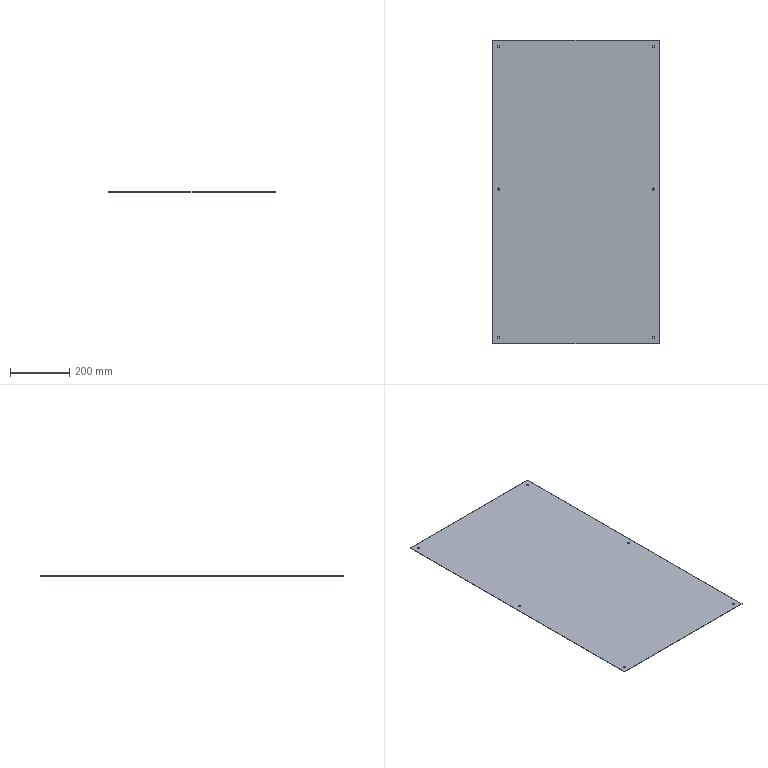Part | SolidWorks | features FlatPattern 1, HoleWzd 1, SMBaseFlange 1, SheetMetal 1 | 1 solid | 18 faces | box 560 x 1020 x 1.2 mm | volume 685163 mm3 | cylinder 12 | plane 6 | commonest cylinder face diameters 7 x12
STEP:
#1=CARTESIAN_POINT('',(16.5,-1000.,0.));
#2=VERTEX_POINT('',#1);
#3=CARTESIAN_POINT('',(23.5,-1000.,0.));
#4=VERTEX_POINT('',#3);
#5=CARTESIAN_POINT('',(20.,-1000.,0.));
#6=DIRECTION('',(0.,0.,1.));
#7=DIRECTION('',(1.,0.,0.));
#8=AXIS2_PLACEMENT_3D('',#5,#6,#7);
#9=CIRCLE('',#8,3.5);
#10=EDGE_CURVE('',#2,#4,#9,.T.);
#11=ORIENTED_EDGE('',*,*,#10,.F.);
#12=CARTESIAN_POINT('',(16.5,-1000.,1.2));
#13=VERTEX_POINT('',#12);
#14=CARTESIAN_POINT('',(16.5,-1000.,1.2));
#15=DIRECTION('',(0.,0.,1.));
#16=VECTOR('',#15,1000.);
#17=LINE('',#14,#16);
#18=EDGE_CURVE('',#2,#13,#17,.T.);
#19=ORIENTED_EDGE('',*,*,#18,.T.);
#20=CARTESIAN_POINT('',(23.5,-1000.,1.2));
#21=VERTEX_POINT('',#20);
#22=CARTESIAN_POINT('',(20.,-1000.,1.2));
#23=DIRECTION('',(0.,0.,1.));
#24=DIRECTION('',(1.,0.,0.));
#25=AXIS2_PLACEMENT_3D('',#22,#23,#24);
#26=CIRCLE('',#25,3.5);
#27=EDGE_CURVE('',#13,#21,#26,.T.);
#28=ORIENTED_EDGE('',*,*,#27,.T.);
#29=CARTESIAN_POINT('',(23.5,-1000.,1.2));
#30=DIRECTION('',(0.,0.,1.));
#31=VECTOR('',#30,1000.);
#32=LINE('',#29,#31);
#33=EDGE_CURVE('',#4,#21,#32,.T.);
#34=ORIENTED_EDGE('',*,*,#33,.F.);
#35=EDGE_LOOP('',(#11,#19,#28,#34));
#36=FACE_OUTER_BOUND('',#35,.T.);
#37=CARTESIAN_POINT('',(20.,-1000.,1.2));
#38=DIRECTION('',(0.,0.,1.));
#39=DIRECTION('',(1.,0.,0.));
#40=AXIS2_PLACEMENT_3D('',#37,#38,#39);
#41=CYLINDRICAL_SURFACE('',#40,3.5);
#42=ADVANCED_FACE('',(#36),#41,.F.);
#43=CARTESIAN_POINT('',(536.5,-1000.,0.));
#44=VERTEX_POINT('',#43);
#45=CARTESIAN_POINT('',(543.5,-1000.,0.));
#46=VERTEX_POINT('',#45);
#47=CARTESIAN_POINT('',(540.,-1000.,0.));
#48=DIRECTION('',(0.,0.,1.));
#49=DIRECTION('',(1.,0.,0.));
#50=AXIS2_PLACEMENT_3D('',#47,#48,#49);
#51=CIRCLE('',#50,3.5);
#52=EDGE_CURVE('',#44,#46,#51,.T.);
#53=ORIENTED_EDGE('',*,*,#52,.F.);
#54=CARTESIAN_POINT('',(536.5,-1000.,1.2));
#55=VERTEX_POINT('',#54);
#56=CARTESIAN_POINT('',(536.5,-1000.,1.2));
#57=DIRECTION('',(0.,0.,1.));
#58=VECTOR('',#57,1000.);
#59=LINE('',#56,#58);
#60=EDGE_CURVE('',#44,#55,#59,.T.);
#61=ORIENTED_EDGE('',*,*,#60,.T.);
#62=CARTESIAN_POINT('',(543.5,-1000.,1.2));
#63=VERTEX_POINT('',#62);
#64=CARTESIAN_POINT('',(540.,-1000.,1.2));
#65=DIRECTION('',(0.,0.,1.));
#66=DIRECTION('',(1.,0.,0.));
#67=AXIS2_PLACEMENT_3D('',#64,#65,#66);
#68=CIRCLE('',#67,3.5);
#69=EDGE_CURVE('',#55,#63,#68,.T.);
#70=ORIENTED_EDGE('',*,*,#69,.T.);
#71=CARTESIAN_POINT('',(543.5,-1000.,1.2));
#72=DIRECTION('',(0.,0.,1.));
#73=VECTOR('',#72,1000.);
#74=LINE('',#71,#73);
#75=EDGE_CURVE('',#46,#63,#74,.T.);
#76=ORIENTED_EDGE('',*,*,#75,.F.);
#77=EDGE_LOOP('',(#53,#61,#70,#76));
#78=FACE_OUTER_BOUND('',#77,.T.);
#79=CARTESIAN_POINT('',(540.,-1000.,1.2));
#80=DIRECTION('',(0.,0.,1.));
#81=DIRECTION('',(1.,0.,0.));
#82=AXIS2_PLACEMENT_3D('',#79,#80,#81);
#83=CYLINDRICAL_SURFACE('',#82,3.5);
#84=ADVANCED_FACE('',(#78),#83,.F.);
#85=CARTESIAN_POINT('',(536.5,-500.,0.));
#86=VERTEX_POINT('',#85);
#87=CARTESIAN_POINT('',(543.5,-500.,0.));
#88=VERTEX_POINT('',#87);
#89=CARTESIAN_POINT('',(540.,-500.,0.));
#90=DIRECTION('',(0.,0.,1.));
#91=DIRECTION('',(1.,0.,0.));
#92=AXIS2_PLACEMENT_3D('',#89,#90,#91);
#93=CIRCLE('',#92,3.5);
#94=EDGE_CURVE('',#86,#88,#93,.T.);
#95=ORIENTED_EDGE('',*,*,#94,.F.);
#96=CARTESIAN_POINT('',(536.5,-500.,1.2));
#97=VERTEX_POINT('',#96);
#98=CARTESIAN_POINT('',(536.5,-500.,1.2));
#99=DIRECTION('',(0.,0.,1.));
#100=VECTOR('',#99,1000.);
#101=LINE('',#98,#100);
#102=EDGE_CURVE('',#86,#97,#101,.T.);
#103=ORIENTED_EDGE('',*,*,#102,.T.);
#104=CARTESIAN_POINT('',(543.5,-500.,1.2));
#105=VERTEX_POINT('',#104);
#106=CARTESIAN_POINT('',(540.,-500.,1.2));
#107=DIRECTION('',(0.,0.,1.));
#108=DIRECTION('',(1.,0.,0.));
#109=AXIS2_PLACEMENT_3D('',#106,#107,#108);
#110=CIRCLE('',#109,3.5);
#111=EDGE_CURVE('',#97,#105,#110,.T.);
#112=ORIENTED_EDGE('',*,*,#111,.T.);
#113=CARTESIAN_POINT('',(543.5,-500.,1.2));
#114=DIRECTION('',(0.,0.,1.));
#115=VECTOR('',#114,1000.);
#116=LINE('',#113,#115);
#117=EDGE_CURVE('',#88,#105,#116,.T.);
#118=ORIENTED_EDGE('',*,*,#117,.F.);
#119=EDGE_LOOP('',(#95,#103,#112,#118));
#120=FACE_OUTER_BOUND('',#119,.T.);
#121=CARTESIAN_POINT('',(540.,-500.,1.2));
#122=DIRECTION('',(0.,0.,1.));
#123=DIRECTION('',(1.,0.,0.));
#124=AXIS2_PLACEMENT_3D('',#121,#122,#123);
#125=CYLINDRICAL_SURFACE('',#124,3.5);
#126=ADVANCED_FACE('',(#120),#125,.F.);
#127=CARTESIAN_POINT('',(16.5,-500.,0.));
#128=VERTEX_POINT('',#127);
#129=CARTESIAN_POINT('',(23.5,-500.,0.));
#130=VERTEX_POINT('',#129);
#131=CARTESIAN_POINT('',(20.,-500.,0.));
#132=DIRECTION('',(0.,0.,1.));
#133=DIRECTION('',(1.,0.,0.));
#134=AXIS2_PLACEMENT_3D('',#131,#132,#133);
#135=CIRCLE('',#134,3.5);
#136=EDGE_CURVE('',#128,#130,#135,.T.);
#137=ORIENTED_EDGE('',*,*,#136,.F.);
#138=CARTESIAN_POINT('',(16.5,-500.,1.2));
#139=VERTEX_POINT('',#138);
#140=CARTESIAN_POINT('',(16.5,-500.,1.2));
#141=DIRECTION('',(0.,0.,1.));
#142=VECTOR('',#141,1000.);
#143=LINE('',#140,#142);
#144=EDGE_CURVE('',#128,#139,#143,.T.);
#145=ORIENTED_EDGE('',*,*,#144,.T.);
#146=CARTESIAN_POINT('',(23.5,-500.,1.2));
#147=VERTEX_POINT('',#146);
#148=CARTESIAN_POINT('',(20.,-500.,1.2));
#149=DIRECTION('',(0.,0.,1.));
#150=DIRECTION('',(1.,0.,0.));
#151=AXIS2_PLACEMENT_3D('',#148,#149,#150);
#152=CIRCLE('',#151,3.5);
#153=EDGE_CURVE('',#139,#147,#152,.T.);
#154=ORIENTED_EDGE('',*,*,#153,.T.);
#155=CARTESIAN_POINT('',(23.5,-500.,1.2));
#156=DIRECTION('',(0.,0.,1.));
#157=VECTOR('',#156,1000.);
#158=LINE('',#155,#157);
#159=EDGE_CURVE('',#130,#147,#158,.T.);
#160=ORIENTED_EDGE('',*,*,#159,.F.);
#161=EDGE_LOOP('',(#137,#145,#154,#160));
#162=FACE_OUTER_BOUND('',#161,.T.);
#163=CARTESIAN_POINT('',(20.,-500.,1.2));
#164=DIRECTION('',(0.,0.,1.));
#165=DIRECTION('',(1.,0.,0.));
#166=AXIS2_PLACEMENT_3D('',#163,#164,#165);
#167=CYLINDRICAL_SURFACE('',#166,3.5);
#168=ADVANCED_FACE('',(#162),#167,.F.);
#169=CARTESIAN_POINT('',(536.5,-20.,0.));
#170=VERTEX_POINT('',#169);
#171=CARTESIAN_POINT('',(543.5,-20.,0.));
#172=VERTEX_POINT('',#171);
#173=CARTESIAN_POINT('',(540.,-20.,0.));
#174=DIRECTION('',(0.,0.,1.));
#175=DIRECTION('',(1.,0.,0.));
#176=AXIS2_PLACEMENT_3D('',#173,#174,#175);
#177=CIRCLE('',#176,3.5);
#178=EDGE_CURVE('',#170,#172,#177,.T.);
#179=ORIENTED_EDGE('',*,*,#178,.F.);
#180=CARTESIAN_POINT('',(536.5,-20.,1.2));
#181=VERTEX_POINT('',#180);
#182=CARTESIAN_POINT('',(536.5,-20.,1.2));
#183=DIRECTION('',(0.,0.,1.));
#184=VECTOR('',#183,1000.);
#185=LINE('',#182,#184);
#186=EDGE_CURVE('',#170,#181,#185,.T.);
#187=ORIENTED_EDGE('',*,*,#186,.T.);
#188=CARTESIAN_POINT('',(543.5,-20.,1.2));
#189=VERTEX_POINT('',#188);
#190=CARTESIAN_POINT('',(540.,-20.,1.2));
#191=DIRECTION('',(0.,0.,1.));
#192=DIRECTION('',(1.,0.,0.));
#193=AXIS2_PLACEMENT_3D('',#190,#191,#192);
#194=CIRCLE('',#193,3.5);
#195=EDGE_CURVE('',#181,#189,#194,.T.);
#196=ORIENTED_EDGE('',*,*,#195,.T.);
#197=CARTESIAN_POINT('',(543.5,-20.,1.2));
#198=DIRECTION('',(0.,0.,1.));
#199=VECTOR('',#198,1000.);
#200=LINE('',#197,#199);
#201=EDGE_CURVE('',#172,#189,#200,.T.);
#202=ORIENTED_EDGE('',*,*,#201,.F.);
#203=EDGE_LOOP('',(#179,#187,#196,#202));
#204=FACE_OUTER_BOUND('',#203,.T.);
#205=CARTESIAN_POINT('',(540.,-20.,1.2));
#206=DIRECTION('',(0.,0.,1.));
#207=DIRECTION('',(1.,0.,0.));
#208=AXIS2_PLACEMENT_3D('',#205,#206,#207);
#209=CYLINDRICAL_SURFACE('',#208,3.5);
#210=ADVANCED_FACE('',(#204),#209,.F.);
#211=CARTESIAN_POINT('',(16.5,-20.,0.));
#212=VERTEX_POINT('',#211);
#213=CARTESIAN_POINT('',(23.5,-20.,0.));
#214=VERTEX_POINT('',#213);
#215=CARTESIAN_POINT('',(20.,-20.,0.));
#216=DIRECTION('',(0.,0.,1.));
#217=DIRECTION('',(1.,0.,0.));
#218=AXIS2_PLACEMENT_3D('',#215,#216,#217);
#219=CIRCLE('',#218,3.5);
#220=EDGE_CURVE('',#212,#214,#219,.T.);
#221=ORIENTED_EDGE('',*,*,#220,.F.);
#222=CARTESIAN_POINT('',(16.5,-20.,1.2));
#223=VERTEX_POINT('',#222);
#224=CARTESIAN_POINT('',(16.5,-20.,1.2));
#225=DIRECTION('',(0.,0.,1.));
#226=VECTOR('',#225,1000.);
#227=LINE('',#224,#226);
#228=EDGE_CURVE('',#212,#223,#227,.T.);
#229=ORIENTED_EDGE('',*,*,#228,.T.);
#230=CARTESIAN_POINT('',(23.5,-20.,1.2));
#231=VERTEX_POINT('',#230);
#232=CARTESIAN_POINT('',(20.,-20.,1.2));
#233=DIRECTION('',(0.,0.,1.));
#234=DIRECTION('',(1.,0.,0.));
#235=AXIS2_PLACEMENT_3D('',#232,#233,#234);
#236=CIRCLE('',#235,3.5);
#237=EDGE_CURVE('',#223,#231,#236,.T.);
#238=ORIENTED_EDGE('',*,*,#237,.T.);
#239=CARTESIAN_POINT('',(23.5,-20.,1.2));
#240=DIRECTION('',(0.,0.,1.));
#241=VECTOR('',#240,1000.);
#242=LINE('',#239,#241);
#243=EDGE_CURVE('',#214,#231,#242,.T.);
#244=ORIENTED_EDGE('',*,*,#243,.F.);
#245=EDGE_LOOP('',(#221,#229,#238,#244));
#246=FACE_OUTER_BOUND('',#245,.T.);
#247=CARTESIAN_POINT('',(20.,-20.,1.2));
#248=DIRECTION('',(0.,0.,1.));
#249=DIRECTION('',(1.,0.,0.));
#250=AXIS2_PLACEMENT_3D('',#247,#248,#249);
#251=CYLINDRICAL_SURFACE('',#250,3.5);
#252=ADVANCED_FACE('',(#246),#251,.F.);
#253=CARTESIAN_POINT('',(0.,-1020.,0.));
#254=VERTEX_POINT('',#253);
#255=CARTESIAN_POINT('',(0.,0.,0.));
#256=VERTEX_POINT('',#255);
#257=CARTESIAN_POINT('',(0.,0.,0.));
#258=DIRECTION('',(0.,1.,0.));
#259=VECTOR('',#258,1000.);
#260=LINE('',#257,#259);
#261=EDGE_CURVE('',#254,#256,#260,.T.);
#262=ORIENTED_EDGE('',*,*,#261,.F.);
#263=CARTESIAN_POINT('',(0.,-1020.,1.2));
#264=VERTEX_POINT('',#263);
#265=CARTESIAN_POINT('',(0.,-1020.,1.2));
#266=DIRECTION('',(0.,0.,-1.));
#267=VECTOR('',#266,1000.);
#268=LINE('',#265,#267);
#269=EDGE_CURVE('',#264,#254,#268,.T.);
#270=ORIENTED_EDGE('',*,*,#269,.F.);
#271=CARTESIAN_POINT('',(0.,0.,1.2));
#272=VERTEX_POINT('',#271);
#273=CARTESIAN_POINT('',(0.,0.,1.2));
#274=DIRECTION('',(0.,1.,0.));
#275=VECTOR('',#274,1000.);
#276=LINE('',#273,#275);
#277=EDGE_CURVE('',#264,#272,#276,.T.);
#278=ORIENTED_EDGE('',*,*,#277,.T.);
#279=CARTESIAN_POINT('',(0.,0.,1.2));
#280=DIRECTION('',(0.,0.,-1.));
#281=VECTOR('',#280,1000.);
#282=LINE('',#279,#281);
#283=EDGE_CURVE('',#272,#256,#282,.T.);
#284=ORIENTED_EDGE('',*,*,#283,.T.);
#285=EDGE_LOOP('',(#262,#270,#278,#284));
#286=FACE_OUTER_BOUND('',#285,.T.);
#287=CARTESIAN_POINT('',(0.,0.,1.2));
#288=DIRECTION('',(-1.,0.,0.));
#289=DIRECTION('',(0.,0.,1.));
#290=AXIS2_PLACEMENT_3D('',#287,#288,#289);
#291=PLANE('',#290);
#292=ADVANCED_FACE('',(#286),#291,.T.);
#293=CARTESIAN_POINT('',(560.,-1020.,0.));
#294=VERTEX_POINT('',#293);
#295=CARTESIAN_POINT('',(0.,-1020.,0.));
#296=DIRECTION('',(-1.,0.,0.));
#297=VECTOR('',#296,1000.);
#298=LINE('',#295,#297);
#299=EDGE_CURVE('',#294,#254,#298,.T.);
#300=ORIENTED_EDGE('',*,*,#299,.F.);
#301=CARTESIAN_POINT('',(560.,-1020.,1.2));
#302=VERTEX_POINT('',#301);
#303=CARTESIAN_POINT('',(560.,-1020.,1.2));
#304=DIRECTION('',(0.,0.,-1.));
#305=VECTOR('',#304,1000.);
#306=LINE('',#303,#305);
#307=EDGE_CURVE('',#302,#294,#306,.T.);
#308=ORIENTED_EDGE('',*,*,#307,.F.);
#309=CARTESIAN_POINT('',(0.,-1020.,1.2));
#310=DIRECTION('',(-1.,0.,0.));
#311=VECTOR('',#310,1000.);
#312=LINE('',#309,#311);
#313=EDGE_CURVE('',#302,#264,#312,.T.);
#314=ORIENTED_EDGE('',*,*,#313,.T.);
#315=ORIENTED_EDGE('',*,*,#269,.T.);
#316=EDGE_LOOP('',(#300,#308,#314,#315));
#317=FACE_OUTER_BOUND('',#316,.T.);
#318=CARTESIAN_POINT('',(0.,-1020.,1.2));
#319=DIRECTION('',(0.,-1.,0.));
#320=DIRECTION('',(0.,0.,-1.));
#321=AXIS2_PLACEMENT_3D('',#318,#319,#320);
#322=PLANE('',#321);
#323=ADVANCED_FACE('',(#317),#322,.T.);
#324=CARTESIAN_POINT('',(560.,0.,0.));
#325=VERTEX_POINT('',#324);
#326=CARTESIAN_POINT('',(560.,0.,0.));
#327=DIRECTION('',(0.,-1.,0.));
#328=VECTOR('',#327,1000.);
#329=LINE('',#326,#328);
#330=EDGE_CURVE('',#325,#294,#329,.T.);
#331=ORIENTED_EDGE('',*,*,#330,.F.);
#332=CARTESIAN_POINT('',(560.,0.,1.2));
#333=VERTEX_POINT('',#332);
#334=CARTESIAN_POINT('',(560.,0.,1.2));
#335=DIRECTION('',(0.,0.,-1.));
#336=VECTOR('',#335,1000.);
#337=LINE('',#334,#336);
#338=EDGE_CURVE('',#333,#325,#337,.T.);
#339=ORIENTED_EDGE('',*,*,#338,.F.);
#340=CARTESIAN_POINT('',(560.,0.,1.2));
#341=DIRECTION('',(0.,-1.,0.));
#342=VECTOR('',#341,1000.);
#343=LINE('',#340,#342);
#344=EDGE_CURVE('',#333,#302,#343,.T.);
#345=ORIENTED_EDGE('',*,*,#344,.T.);
#346=ORIENTED_EDGE('',*,*,#307,.T.);
#347=EDGE_LOOP('',(#331,#339,#345,#346));
#348=FACE_OUTER_BOUND('',#347,.T.);
#349=CARTESIAN_POINT('',(560.,0.,1.2));
#350=DIRECTION('',(1.,0.,0.));
#351=DIRECTION('',(0.,0.,-1.));
#352=AXIS2_PLACEMENT_3D('',#349,#350,#351);
#353=PLANE('',#352);
#354=ADVANCED_FACE('',(#348),#353,.T.);
#355=CARTESIAN_POINT('',(0.,0.,0.));
#356=DIRECTION('',(1.,0.,0.));
#357=VECTOR('',#356,1000.);
#358=LINE('',#355,#357);
#359=EDGE_CURVE('',#256,#325,#358,.T.);
#360=ORIENTED_EDGE('',*,*,#359,.F.);
#361=ORIENTED_EDGE('',*,*,#283,.F.);
#362=CARTESIAN_POINT('',(0.,0.,1.2));
#363=DIRECTION('',(1.,0.,0.));
#364=VECTOR('',#363,1000.);
#365=LINE('',#362,#364);
#366=EDGE_CURVE('',#272,#333,#365,.T.);
#367=ORIENTED_EDGE('',*,*,#366,.T.);
#368=ORIENTED_EDGE('',*,*,#338,.T.);
#369=EDGE_LOOP('',(#360,#361,#367,#368));
#370=FACE_OUTER_BOUND('',#369,.T.);
#371=CARTESIAN_POINT('',(0.,0.,1.2));
#372=DIRECTION('',(0.,1.,0.));
#373=DIRECTION('',(0.,0.,1.));
#374=AXIS2_PLACEMENT_3D('',#371,#372,#373);
#375=PLANE('',#374);
#376=ADVANCED_FACE('',(#370),#375,.T.);
#377=CARTESIAN_POINT('',(20.,-1000.,1.2));
#378=DIRECTION('',(0.,0.,1.));
#379=DIRECTION('',(1.,0.,0.));
#380=AXIS2_PLACEMENT_3D('',#377,#378,#379);
#381=CIRCLE('',#380,3.5);
#382=EDGE_CURVE('',#21,#13,#381,.T.);
#383=ORIENTED_EDGE('',*,*,#382,.F.);
#384=ORIENTED_EDGE('',*,*,#27,.F.);
#385=EDGE_LOOP('',(#383,#384));
#386=FACE_BOUND('',#385,.T.);
#387=CARTESIAN_POINT('',(540.,-1000.,1.2));
#388=DIRECTION('',(0.,0.,1.));
#389=DIRECTION('',(1.,0.,0.));
#390=AXIS2_PLACEMENT_3D('',#387,#388,#389);
#391=CIRCLE('',#390,3.5);
#392=EDGE_CURVE('',#63,#55,#391,.T.);
#393=ORIENTED_EDGE('',*,*,#392,.F.);
#394=ORIENTED_EDGE('',*,*,#69,.F.);
#395=EDGE_LOOP('',(#393,#394));
#396=FACE_BOUND('',#395,.T.);
#397=CARTESIAN_POINT('',(540.,-500.,1.2));
#398=DIRECTION('',(0.,0.,1.));
#399=DIRECTION('',(1.,0.,0.));
#400=AXIS2_PLACEMENT_3D('',#397,#398,#399);
#401=CIRCLE('',#400,3.5);
#402=EDGE_CURVE('',#105,#97,#401,.T.);
#403=ORIENTED_EDGE('',*,*,#402,.F.);
#404=ORIENTED_EDGE('',*,*,#111,.F.);
#405=EDGE_LOOP('',(#403,#404));
#406=FACE_BOUND('',#405,.T.);
#407=CARTESIAN_POINT('',(20.,-500.,1.2));
#408=DIRECTION('',(0.,0.,1.));
#409=DIRECTION('',(1.,0.,0.));
#410=AXIS2_PLACEMENT_3D('',#407,#408,#409);
#411=CIRCLE('',#410,3.5);
#412=EDGE_CURVE('',#147,#139,#411,.T.);
#413=ORIENTED_EDGE('',*,*,#412,.F.);
#414=ORIENTED_EDGE('',*,*,#153,.F.);
#415=EDGE_LOOP('',(#413,#414));
#416=FACE_BOUND('',#415,.T.);
#417=CARTESIAN_POINT('',(540.,-20.,1.2));
#418=DIRECTION('',(0.,0.,1.));
#419=DIRECTION('',(1.,0.,0.));
#420=AXIS2_PLACEMENT_3D('',#417,#418,#419);
#421=CIRCLE('',#420,3.5);
#422=EDGE_CURVE('',#189,#181,#421,.T.);
#423=ORIENTED_EDGE('',*,*,#422,.F.);
#424=ORIENTED_EDGE('',*,*,#195,.F.);
#425=EDGE_LOOP('',(#423,#424));
#426=FACE_BOUND('',#425,.T.);
#427=CARTESIAN_POINT('',(20.,-20.,1.2));
#428=DIRECTION('',(0.,0.,1.));
#429=DIRECTION('',(1.,0.,0.));
#430=AXIS2_PLACEMENT_3D('',#427,#428,#429);
#431=CIRCLE('',#430,3.5);
#432=EDGE_CURVE('',#231,#223,#431,.T.);
#433=ORIENTED_EDGE('',*,*,#432,.F.);
#434=ORIENTED_EDGE('',*,*,#237,.F.);
#435=EDGE_LOOP('',(#433,#434));
#436=FACE_BOUND('',#435,.T.);
#437=ORIENTED_EDGE('',*,*,#277,.F.);
#438=ORIENTED_EDGE('',*,*,#313,.F.);
#439=ORIENTED_EDGE('',*,*,#344,.F.);
#440=ORIENTED_EDGE('',*,*,#366,.F.);
#441=EDGE_LOOP('',(#437,#438,#439,#440));
#442=FACE_OUTER_BOUND('',#441,.T.);
#443=CARTESIAN_POINT('',(0.,0.,1.2));
#444=DIRECTION('',(0.,0.,1.));
#445=DIRECTION('',(1.,0.,0.));
#446=AXIS2_PLACEMENT_3D('',#443,#444,#445);
#447=PLANE('',#446);
#448=ADVANCED_FACE('',(#386,#396,#406,#416,#426,#436,#442),#447,.T.);
#449=CARTESIAN_POINT('',(20.,-1000.,0.));
#450=DIRECTION('',(0.,0.,1.));
#451=DIRECTION('',(1.,0.,0.));
#452=AXIS2_PLACEMENT_3D('',#449,#450,#451);
#453=CIRCLE('',#452,3.5);
#454=EDGE_CURVE('',#4,#2,#453,.T.);
#455=ORIENTED_EDGE('',*,*,#454,.T.);
#456=ORIENTED_EDGE('',*,*,#10,.T.);
#457=EDGE_LOOP('',(#455,#456));
#458=FACE_BOUND('',#457,.T.);
#459=CARTESIAN_POINT('',(540.,-1000.,0.));
#460=DIRECTION('',(0.,0.,1.));
#461=DIRECTION('',(1.,0.,0.));
#462=AXIS2_PLACEMENT_3D('',#459,#460,#461);
#463=CIRCLE('',#462,3.5);
#464=EDGE_CURVE('',#46,#44,#463,.T.);
#465=ORIENTED_EDGE('',*,*,#464,.T.);
#466=ORIENTED_EDGE('',*,*,#52,.T.);
#467=EDGE_LOOP('',(#465,#466));
#468=FACE_BOUND('',#467,.T.);
#469=CARTESIAN_POINT('',(540.,-500.,0.));
#470=DIRECTION('',(0.,0.,1.));
#471=DIRECTION('',(1.,0.,0.));
#472=AXIS2_PLACEMENT_3D('',#469,#470,#471);
#473=CIRCLE('',#472,3.5);
#474=EDGE_CURVE('',#88,#86,#473,.T.);
#475=ORIENTED_EDGE('',*,*,#474,.T.);
#476=ORIENTED_EDGE('',*,*,#94,.T.);
#477=EDGE_LOOP('',(#475,#476));
#478=FACE_BOUND('',#477,.T.);
#479=CARTESIAN_POINT('',(20.,-500.,0.));
#480=DIRECTION('',(0.,0.,1.));
#481=DIRECTION('',(1.,0.,0.));
#482=AXIS2_PLACEMENT_3D('',#479,#480,#481);
#483=CIRCLE('',#482,3.5);
#484=EDGE_CURVE('',#130,#128,#483,.T.);
#485=ORIENTED_EDGE('',*,*,#484,.T.);
#486=ORIENTED_EDGE('',*,*,#136,.T.);
#487=EDGE_LOOP('',(#485,#486));
#488=FACE_BOUND('',#487,.T.);
#489=CARTESIAN_POINT('',(540.,-20.,0.));
#490=DIRECTION('',(0.,0.,1.));
#491=DIRECTION('',(1.,0.,0.));
#492=AXIS2_PLACEMENT_3D('',#489,#490,#491);
#493=CIRCLE('',#492,3.5);
#494=EDGE_CURVE('',#172,#170,#493,.T.);
#495=ORIENTED_EDGE('',*,*,#494,.T.);
#496=ORIENTED_EDGE('',*,*,#178,.T.);
#497=EDGE_LOOP('',(#495,#496));
#498=FACE_BOUND('',#497,.T.);
#499=CARTESIAN_POINT('',(20.,-20.,0.));
#500=DIRECTION('',(0.,0.,1.));
#501=DIRECTION('',(1.,0.,0.));
#502=AXIS2_PLACEMENT_3D('',#499,#500,#501);
#503=CIRCLE('',#502,3.5);
#504=EDGE_CURVE('',#214,#212,#503,.T.);
#505=ORIENTED_EDGE('',*,*,#504,.T.);
#506=ORIENTED_EDGE('',*,*,#220,.T.);
#507=EDGE_LOOP('',(#505,#506));
#508=FACE_BOUND('',#507,.T.);
#509=ORIENTED_EDGE('',*,*,#261,.T.);
#510=ORIENTED_EDGE('',*,*,#359,.T.);
#511=ORIENTED_EDGE('',*,*,#330,.T.);
#512=ORIENTED_EDGE('',*,*,#299,.T.);
#513=EDGE_LOOP('',(#509,#510,#511,#512));
#514=FACE_OUTER_BOUND('',#513,.T.);
#515=CARTESIAN_POINT('',(0.,0.,0.));
#516=DIRECTION('',(0.,0.,1.));
#517=DIRECTION('',(1.,0.,0.));
#518=AXIS2_PLACEMENT_3D('',#515,#516,#517);
#519=PLANE('',#518);
#520=ADVANCED_FACE('',(#458,#468,#478,#488,#498,#508,#514),#519,.F.);
#521=ORIENTED_EDGE('',*,*,#228,.F.);
#522=ORIENTED_EDGE('',*,*,#504,.F.);
#523=ORIENTED_EDGE('',*,*,#243,.T.);
#524=ORIENTED_EDGE('',*,*,#432,.T.);
#525=EDGE_LOOP('',(#521,#522,#523,#524));
#526=FACE_OUTER_BOUND('',#525,.T.);
#527=CARTESIAN_POINT('',(20.,-20.,1.2));
#528=DIRECTION('',(0.,0.,1.));
#529=DIRECTION('',(1.,0.,0.));
#530=AXIS2_PLACEMENT_3D('',#527,#528,#529);
#531=CYLINDRICAL_SURFACE('',#530,3.5);
#532=ADVANCED_FACE('',(#526),#531,.F.);
#533=ORIENTED_EDGE('',*,*,#186,.F.);
#534=ORIENTED_EDGE('',*,*,#494,.F.);
#535=ORIENTED_EDGE('',*,*,#201,.T.);
#536=ORIENTED_EDGE('',*,*,#422,.T.);
#537=EDGE_LOOP('',(#533,#534,#535,#536));
#538=FACE_OUTER_BOUND('',#537,.T.);
#539=CARTESIAN_POINT('',(540.,-20.,1.2));
#540=DIRECTION('',(0.,0.,1.));
#541=DIRECTION('',(1.,0.,0.));
#542=AXIS2_PLACEMENT_3D('',#539,#540,#541);
#543=CYLINDRICAL_SURFACE('',#542,3.5);
#544=ADVANCED_FACE('',(#538),#543,.F.);
#545=ORIENTED_EDGE('',*,*,#144,.F.);
#546=ORIENTED_EDGE('',*,*,#484,.F.);
#547=ORIENTED_EDGE('',*,*,#159,.T.);
#548=ORIENTED_EDGE('',*,*,#412,.T.);
#549=EDGE_LOOP('',(#545,#546,#547,#548));
#550=FACE_OUTER_BOUND('',#549,.T.);
#551=CARTESIAN_POINT('',(20.,-500.,1.2));
#552=DIRECTION('',(0.,0.,1.));
#553=DIRECTION('',(1.,0.,0.));
#554=AXIS2_PLACEMENT_3D('',#551,#552,#553);
#555=CYLINDRICAL_SURFACE('',#554,3.5);
#556=ADVANCED_FACE('',(#550),#555,.F.);
#557=ORIENTED_EDGE('',*,*,#102,.F.);
#558=ORIENTED_EDGE('',*,*,#474,.F.);
#559=ORIENTED_EDGE('',*,*,#117,.T.);
#560=ORIENTED_EDGE('',*,*,#402,.T.);
#561=EDGE_LOOP('',(#557,#558,#559,#560));
#562=FACE_OUTER_BOUND('',#561,.T.);
#563=CARTESIAN_POINT('',(540.,-500.,1.2));
#564=DIRECTION('',(0.,0.,1.));
#565=DIRECTION('',(1.,0.,0.));
#566=AXIS2_PLACEMENT_3D('',#563,#564,#565);
#567=CYLINDRICAL_SURFACE('',#566,3.5);
#568=ADVANCED_FACE('',(#562),#567,.F.);
#569=ORIENTED_EDGE('',*,*,#60,.F.);
#570=ORIENTED_EDGE('',*,*,#464,.F.);
#571=ORIENTED_EDGE('',*,*,#75,.T.);
#572=ORIENTED_EDGE('',*,*,#392,.T.);
#573=EDGE_LOOP('',(#569,#570,#571,#572));
#574=FACE_OUTER_BOUND('',#573,.T.);
#575=CARTESIAN_POINT('',(540.,-1000.,1.2));
#576=DIRECTION('',(0.,0.,1.));
#577=DIRECTION('',(1.,0.,0.));
#578=AXIS2_PLACEMENT_3D('',#575,#576,#577);
#579=CYLINDRICAL_SURFACE('',#578,3.5);
#580=ADVANCED_FACE('',(#574),#579,.F.);
#581=ORIENTED_EDGE('',*,*,#18,.F.);
#582=ORIENTED_EDGE('',*,*,#454,.F.);
#583=ORIENTED_EDGE('',*,*,#33,.T.);
#584=ORIENTED_EDGE('',*,*,#382,.T.);
#585=EDGE_LOOP('',(#581,#582,#583,#584));
#586=FACE_OUTER_BOUND('',#585,.T.);
#587=CARTESIAN_POINT('',(20.,-1000.,1.2));
#588=DIRECTION('',(0.,0.,1.));
#589=DIRECTION('',(1.,0.,0.));
#590=AXIS2_PLACEMENT_3D('',#587,#588,#589);
#591=CYLINDRICAL_SURFACE('',#590,3.5);
#592=ADVANCED_FACE('',(#586),#591,.F.);
#593=CLOSED_SHELL('',(#42,#84,#126,#168,#210,#252,#292,#323,#354,#376,#448,#520,#532,#544,#556,#568,#580,#592));
#594=MANIFOLD_SOLID_BREP('',#593);
#595=CARTESIAN_POINT('',(0.,0.,0.));
#596=DIRECTION('',(0.,0.,1.));
#597=DIRECTION('',(1.,0.,0.));
#598=AXIS2_PLACEMENT_3D('',#595,#596,#597);
#599=(LENGTH_UNIT()NAMED_UNIT(*)SI_UNIT(.MILLI.,.METRE.));
#600=UNCERTAINTY_MEASURE_WITH_UNIT(LENGTH_MEASURE(0.00001),#599,'','');
#601=(NAMED_UNIT(*)PLANE_ANGLE_UNIT()SI_UNIT($,.RADIAN.));
#602=(NAMED_UNIT(*)SI_UNIT($,.STERADIAN.)SOLID_ANGLE_UNIT());
#603=(GEOMETRIC_REPRESENTATION_CONTEXT(3)GLOBAL_UNCERTAINTY_ASSIGNED_CONTEXT((#600))GLOBAL_UNIT_ASSIGNED_CONTEXT((#599,#601,#602))REPRESENTATION_CONTEXT('',''));
#604=ADVANCED_BREP_SHAPE_REPRESENTATION('',(#594,#598),#603);